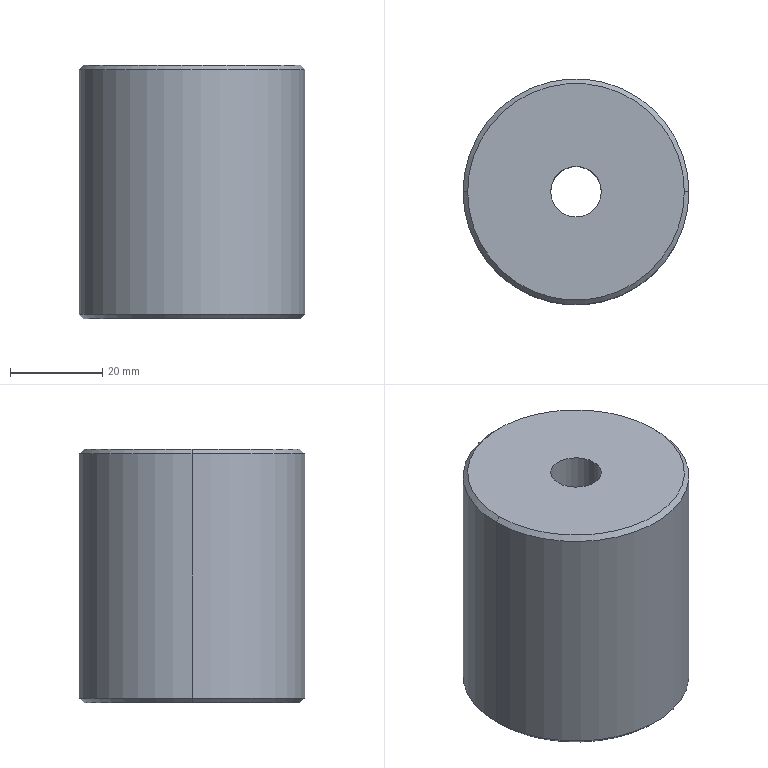Part | SolidWorks | features BaseBody 1 | 1 solid | 13 faces | box 49 x 49 x 55 mm | volume 96424 mm3 | cylinder 6 | cone 4 | plane 3 | commonest cylinder face diameters 11 x2 18 x2 49 x2
STEP:
#1=CARTESIAN_POINT('',(-196.5,115.,-210.5));
#2=VERTEX_POINT('',#1);
#3=CARTESIAN_POINT('',(-243.5,115.,-210.5));
#4=VERTEX_POINT('',#3);
#5=CARTESIAN_POINT('',(-220.,115.,-210.5));
#6=DIRECTION('',(0.,0.,1.));
#7=DIRECTION('',(1.,0.,0.));
#8=AXIS2_PLACEMENT_3D('',#5,#6,#7);
#9=CIRCLE('',#8,23.5);
#10=EDGE_CURVE('',#2,#4,#9,.T.);
#11=ORIENTED_EDGE('',*,*,#10,.F.);
#12=CARTESIAN_POINT('',(-195.5,115.,-211.5));
#13=VERTEX_POINT('',#12);
#14=CARTESIAN_POINT('',(-195.5,115.,-211.5));
#15=DIRECTION('',(0.7071,0.,-0.7071));
#16=VECTOR('',#15,1000.);
#17=LINE('',#14,#16);
#18=EDGE_CURVE('',#2,#13,#17,.T.);
#19=ORIENTED_EDGE('',*,*,#18,.T.);
#20=CARTESIAN_POINT('',(-244.5,115.,-211.5));
#21=VERTEX_POINT('',#20);
#22=CARTESIAN_POINT('',(-220.,115.,-211.5));
#23=DIRECTION('',(0.,0.,-1.));
#24=DIRECTION('',(1.,0.,0.));
#25=AXIS2_PLACEMENT_3D('',#22,#23,#24);
#26=CIRCLE('',#25,24.5);
#27=EDGE_CURVE('',#21,#13,#26,.T.);
#28=ORIENTED_EDGE('',*,*,#27,.F.);
#29=CARTESIAN_POINT('',(-244.5,115.,-211.5));
#30=DIRECTION('',(-0.7071,0.,-0.7071));
#31=VECTOR('',#30,1000.);
#32=LINE('',#29,#31);
#33=EDGE_CURVE('',#4,#21,#32,.T.);
#34=ORIENTED_EDGE('',*,*,#33,.F.);
#35=EDGE_LOOP('',(#11,#19,#28,#34));
#36=FACE_OUTER_BOUND('',#35,.T.);
#37=CARTESIAN_POINT('',(-220.,115.,-211.5));
#38=DIRECTION('',(0.,0.,-1.));
#39=DIRECTION('',(-1.,0.,0.));
#40=AXIS2_PLACEMENT_3D('',#37,#38,#39);
#41=CONICAL_SURFACE('',#40,24.5,0.7854);
#42=ADVANCED_FACE('',(#36),#41,.T.);
#43=CARTESIAN_POINT('',(-243.5,115.,-265.5));
#44=VERTEX_POINT('',#43);
#45=CARTESIAN_POINT('',(-196.5,115.,-265.5));
#46=VERTEX_POINT('',#45);
#47=CARTESIAN_POINT('',(-220.,115.,-265.5));
#48=DIRECTION('',(0.,0.,-1.));
#49=DIRECTION('',(-1.,0.,0.));
#50=AXIS2_PLACEMENT_3D('',#47,#48,#49);
#51=CIRCLE('',#50,23.5);
#52=EDGE_CURVE('',#44,#46,#51,.T.);
#53=ORIENTED_EDGE('',*,*,#52,.F.);
#54=CARTESIAN_POINT('',(-244.5,115.,-264.5));
#55=VERTEX_POINT('',#54);
#56=CARTESIAN_POINT('',(-244.5,115.,-264.5));
#57=DIRECTION('',(-0.7071,0.,0.7071));
#58=VECTOR('',#57,1000.);
#59=LINE('',#56,#58);
#60=EDGE_CURVE('',#44,#55,#59,.T.);
#61=ORIENTED_EDGE('',*,*,#60,.T.);
#62=CARTESIAN_POINT('',(-195.5,115.,-264.5));
#63=VERTEX_POINT('',#62);
#64=CARTESIAN_POINT('',(-220.,115.,-264.5));
#65=DIRECTION('',(0.,0.,1.));
#66=DIRECTION('',(-1.,0.,0.));
#67=AXIS2_PLACEMENT_3D('',#64,#65,#66);
#68=CIRCLE('',#67,24.5);
#69=EDGE_CURVE('',#63,#55,#68,.T.);
#70=ORIENTED_EDGE('',*,*,#69,.F.);
#71=CARTESIAN_POINT('',(-195.5,115.,-264.5));
#72=DIRECTION('',(0.7071,0.,0.7071));
#73=VECTOR('',#72,1000.);
#74=LINE('',#71,#73);
#75=EDGE_CURVE('',#46,#63,#74,.T.);
#76=ORIENTED_EDGE('',*,*,#75,.F.);
#77=EDGE_LOOP('',(#53,#61,#70,#76));
#78=FACE_OUTER_BOUND('',#77,.T.);
#79=CARTESIAN_POINT('',(-220.,115.,-264.5));
#80=DIRECTION('',(0.,0.,1.));
#81=DIRECTION('',(1.,0.,0.));
#82=AXIS2_PLACEMENT_3D('',#79,#80,#81);
#83=CONICAL_SURFACE('',#82,24.5,0.7854);
#84=ADVANCED_FACE('',(#78),#83,.T.);
#85=CARTESIAN_POINT('',(-229.,115.,-265.5));
#86=VERTEX_POINT('',#85);
#87=CARTESIAN_POINT('',(-211.,115.,-265.5));
#88=VERTEX_POINT('',#87);
#89=CARTESIAN_POINT('',(-220.,115.,-265.5));
#90=DIRECTION('',(0.,0.,-1.));
#91=DIRECTION('',(-1.,0.,0.));
#92=AXIS2_PLACEMENT_3D('',#89,#90,#91);
#93=CIRCLE('',#92,9.);
#94=EDGE_CURVE('',#86,#88,#93,.T.);
#95=ORIENTED_EDGE('',*,*,#94,.T.);
#96=CARTESIAN_POINT('',(-211.,115.,-253.5));
#97=VERTEX_POINT('',#96);
#98=CARTESIAN_POINT('',(-211.,115.,-265.5));
#99=DIRECTION('',(0.,0.,1.));
#100=VECTOR('',#99,1000.);
#101=LINE('',#98,#100);
#102=EDGE_CURVE('',#88,#97,#101,.T.);
#103=ORIENTED_EDGE('',*,*,#102,.T.);
#104=CARTESIAN_POINT('',(-229.,115.,-253.5));
#105=VERTEX_POINT('',#104);
#106=CARTESIAN_POINT('',(-220.,115.,-253.5));
#107=DIRECTION('',(0.,0.,-1.));
#108=DIRECTION('',(-1.,0.,0.));
#109=AXIS2_PLACEMENT_3D('',#106,#107,#108);
#110=CIRCLE('',#109,9.);
#111=EDGE_CURVE('',#105,#97,#110,.T.);
#112=ORIENTED_EDGE('',*,*,#111,.F.);
#113=CARTESIAN_POINT('',(-229.,115.,-265.5));
#114=DIRECTION('',(0.,0.,1.));
#115=VECTOR('',#114,1000.);
#116=LINE('',#113,#115);
#117=EDGE_CURVE('',#86,#105,#116,.T.);
#118=ORIENTED_EDGE('',*,*,#117,.F.);
#119=EDGE_LOOP('',(#95,#103,#112,#118));
#120=FACE_OUTER_BOUND('',#119,.T.);
#121=CARTESIAN_POINT('',(-220.,115.,-265.5));
#122=DIRECTION('',(0.,0.,1.));
#123=DIRECTION('',(-1.,0.,0.));
#124=AXIS2_PLACEMENT_3D('',#121,#122,#123);
#125=CYLINDRICAL_SURFACE('',#124,9.);
#126=ADVANCED_FACE('',(#120),#125,.F.);
#127=CARTESIAN_POINT('',(-214.5,115.,-253.5));
#128=VERTEX_POINT('',#127);
#129=CARTESIAN_POINT('',(-225.5,115.,-253.5));
#130=VERTEX_POINT('',#129);
#131=CARTESIAN_POINT('',(-220.,115.,-253.5));
#132=DIRECTION('',(0.,0.,1.));
#133=DIRECTION('',(-1.,0.,0.));
#134=AXIS2_PLACEMENT_3D('',#131,#132,#133);
#135=CIRCLE('',#134,5.5);
#136=EDGE_CURVE('',#128,#130,#135,.T.);
#137=ORIENTED_EDGE('',*,*,#136,.F.);
#138=CARTESIAN_POINT('',(-214.5,115.,-210.5));
#139=VERTEX_POINT('',#138);
#140=CARTESIAN_POINT('',(-214.5,115.,-265.5));
#141=DIRECTION('',(0.,0.,1.));
#142=VECTOR('',#141,1000.);
#143=LINE('',#140,#142);
#144=EDGE_CURVE('',#128,#139,#143,.T.);
#145=ORIENTED_EDGE('',*,*,#144,.T.);
#146=CARTESIAN_POINT('',(-225.5,115.,-210.5));
#147=VERTEX_POINT('',#146);
#148=CARTESIAN_POINT('',(-220.,115.,-210.5));
#149=DIRECTION('',(0.,0.,-1.));
#150=DIRECTION('',(1.,0.,0.));
#151=AXIS2_PLACEMENT_3D('',#148,#149,#150);
#152=CIRCLE('',#151,5.5);
#153=EDGE_CURVE('',#147,#139,#152,.T.);
#154=ORIENTED_EDGE('',*,*,#153,.F.);
#155=CARTESIAN_POINT('',(-225.5,115.,-265.5));
#156=DIRECTION('',(0.,0.,1.));
#157=VECTOR('',#156,1000.);
#158=LINE('',#155,#157);
#159=EDGE_CURVE('',#130,#147,#158,.T.);
#160=ORIENTED_EDGE('',*,*,#159,.F.);
#161=EDGE_LOOP('',(#137,#145,#154,#160));
#162=FACE_OUTER_BOUND('',#161,.T.);
#163=CARTESIAN_POINT('',(-220.,115.,-265.5));
#164=DIRECTION('',(0.,0.,1.));
#165=DIRECTION('',(-1.,0.,0.));
#166=AXIS2_PLACEMENT_3D('',#163,#164,#165);
#167=CYLINDRICAL_SURFACE('',#166,5.5);
#168=ADVANCED_FACE('',(#162),#167,.F.);
#169=CARTESIAN_POINT('',(-220.,115.,-211.5));
#170=DIRECTION('',(0.,0.,-1.));
#171=DIRECTION('',(1.,0.,0.));
#172=AXIS2_PLACEMENT_3D('',#169,#170,#171);
#173=CIRCLE('',#172,24.5);
#174=EDGE_CURVE('',#13,#21,#173,.T.);
#175=ORIENTED_EDGE('',*,*,#174,.T.);
#176=CARTESIAN_POINT('',(-244.5,115.,-165.5));
#177=DIRECTION('',(0.,0.,-1.));
#178=VECTOR('',#177,1000.);
#179=LINE('',#176,#178);
#180=EDGE_CURVE('',#21,#55,#179,.T.);
#181=ORIENTED_EDGE('',*,*,#180,.T.);
#182=CARTESIAN_POINT('',(-220.,115.,-264.5));
#183=DIRECTION('',(0.,0.,1.));
#184=DIRECTION('',(-1.,0.,0.));
#185=AXIS2_PLACEMENT_3D('',#182,#183,#184);
#186=CIRCLE('',#185,24.5);
#187=EDGE_CURVE('',#55,#63,#186,.T.);
#188=ORIENTED_EDGE('',*,*,#187,.T.);
#189=CARTESIAN_POINT('',(-195.5,115.,-165.5));
#190=DIRECTION('',(0.,0.,-1.));
#191=VECTOR('',#190,1000.);
#192=LINE('',#189,#191);
#193=EDGE_CURVE('',#13,#63,#192,.T.);
#194=ORIENTED_EDGE('',*,*,#193,.F.);
#195=EDGE_LOOP('',(#175,#181,#188,#194));
#196=FACE_OUTER_BOUND('',#195,.T.);
#197=CARTESIAN_POINT('',(-220.,115.,-165.5));
#198=DIRECTION('',(0.,0.,-1.));
#199=DIRECTION('',(1.,0.,0.));
#200=AXIS2_PLACEMENT_3D('',#197,#198,#199);
#201=CYLINDRICAL_SURFACE('',#200,24.5);
#202=ADVANCED_FACE('',(#196),#201,.T.);
#203=ORIENTED_EDGE('',*,*,#180,.F.);
#204=ORIENTED_EDGE('',*,*,#27,.T.);
#205=ORIENTED_EDGE('',*,*,#193,.T.);
#206=ORIENTED_EDGE('',*,*,#69,.T.);
#207=EDGE_LOOP('',(#203,#204,#205,#206));
#208=FACE_OUTER_BOUND('',#207,.T.);
#209=CARTESIAN_POINT('',(-220.,115.,-165.5));
#210=DIRECTION('',(0.,0.,-1.));
#211=DIRECTION('',(1.,0.,0.));
#212=AXIS2_PLACEMENT_3D('',#209,#210,#211);
#213=CYLINDRICAL_SURFACE('',#212,24.5);
#214=ADVANCED_FACE('',(#208),#213,.T.);
#215=CARTESIAN_POINT('',(-220.,115.,-210.5));
#216=DIRECTION('',(0.,0.,1.));
#217=DIRECTION('',(1.,0.,0.));
#218=AXIS2_PLACEMENT_3D('',#215,#216,#217);
#219=CIRCLE('',#218,23.5);
#220=EDGE_CURVE('',#4,#2,#219,.T.);
#221=ORIENTED_EDGE('',*,*,#220,.T.);
#222=ORIENTED_EDGE('',*,*,#10,.T.);
#223=EDGE_LOOP('',(#221,#222));
#224=FACE_OUTER_BOUND('',#223,.T.);
#225=ORIENTED_EDGE('',*,*,#153,.T.);
#226=CARTESIAN_POINT('',(-220.,115.,-210.5));
#227=DIRECTION('',(0.,0.,-1.));
#228=DIRECTION('',(1.,0.,0.));
#229=AXIS2_PLACEMENT_3D('',#226,#227,#228);
#230=CIRCLE('',#229,5.5);
#231=EDGE_CURVE('',#139,#147,#230,.T.);
#232=ORIENTED_EDGE('',*,*,#231,.T.);
#233=EDGE_LOOP('',(#225,#232));
#234=FACE_BOUND('',#233,.T.);
#235=CARTESIAN_POINT('',(-170.,-105.,-210.5));
#236=DIRECTION('',(0.,0.,1.));
#237=DIRECTION('',(1.,0.,0.));
#238=AXIS2_PLACEMENT_3D('',#235,#236,#237);
#239=PLANE('',#238);
#240=ADVANCED_FACE('',(#224,#234),#239,.T.);
#241=ORIENTED_EDGE('',*,*,#144,.F.);
#242=CARTESIAN_POINT('',(-220.,115.,-253.5));
#243=DIRECTION('',(0.,0.,1.));
#244=DIRECTION('',(-1.,0.,0.));
#245=AXIS2_PLACEMENT_3D('',#242,#243,#244);
#246=CIRCLE('',#245,5.5);
#247=EDGE_CURVE('',#130,#128,#246,.T.);
#248=ORIENTED_EDGE('',*,*,#247,.F.);
#249=ORIENTED_EDGE('',*,*,#159,.T.);
#250=ORIENTED_EDGE('',*,*,#231,.F.);
#251=EDGE_LOOP('',(#241,#248,#249,#250));
#252=FACE_OUTER_BOUND('',#251,.T.);
#253=CARTESIAN_POINT('',(-220.,115.,-265.5));
#254=DIRECTION('',(0.,0.,1.));
#255=DIRECTION('',(-1.,0.,0.));
#256=AXIS2_PLACEMENT_3D('',#253,#254,#255);
#257=CYLINDRICAL_SURFACE('',#256,5.5);
#258=ADVANCED_FACE('',(#252),#257,.F.);
#259=CARTESIAN_POINT('',(-220.,115.,-265.5));
#260=DIRECTION('',(0.,0.,-1.));
#261=DIRECTION('',(-1.,0.,0.));
#262=AXIS2_PLACEMENT_3D('',#259,#260,#261);
#263=CIRCLE('',#262,23.5);
#264=EDGE_CURVE('',#46,#44,#263,.T.);
#265=ORIENTED_EDGE('',*,*,#264,.T.);
#266=ORIENTED_EDGE('',*,*,#52,.T.);
#267=EDGE_LOOP('',(#265,#266));
#268=FACE_OUTER_BOUND('',#267,.T.);
#269=ORIENTED_EDGE('',*,*,#94,.F.);
#270=CARTESIAN_POINT('',(-220.,115.,-265.5));
#271=DIRECTION('',(0.,0.,-1.));
#272=DIRECTION('',(-1.,0.,0.));
#273=AXIS2_PLACEMENT_3D('',#270,#271,#272);
#274=CIRCLE('',#273,9.);
#275=EDGE_CURVE('',#88,#86,#274,.T.);
#276=ORIENTED_EDGE('',*,*,#275,.F.);
#277=EDGE_LOOP('',(#269,#276));
#278=FACE_BOUND('',#277,.T.);
#279=CARTESIAN_POINT('',(-220.,115.,-265.5));
#280=DIRECTION('',(0.,0.,-1.));
#281=DIRECTION('',(1.,0.,0.));
#282=AXIS2_PLACEMENT_3D('',#279,#280,#281);
#283=PLANE('',#282);
#284=ADVANCED_FACE('',(#268,#278),#283,.T.);
#285=ORIENTED_EDGE('',*,*,#111,.T.);
#286=CARTESIAN_POINT('',(-220.,115.,-253.5));
#287=DIRECTION('',(0.,0.,-1.));
#288=DIRECTION('',(-1.,0.,0.));
#289=AXIS2_PLACEMENT_3D('',#286,#287,#288);
#290=CIRCLE('',#289,9.);
#291=EDGE_CURVE('',#97,#105,#290,.T.);
#292=ORIENTED_EDGE('',*,*,#291,.T.);
#293=EDGE_LOOP('',(#285,#292));
#294=FACE_OUTER_BOUND('',#293,.T.);
#295=ORIENTED_EDGE('',*,*,#247,.T.);
#296=ORIENTED_EDGE('',*,*,#136,.T.);
#297=EDGE_LOOP('',(#295,#296));
#298=FACE_BOUND('',#297,.T.);
#299=CARTESIAN_POINT('',(-220.,115.,-253.5));
#300=DIRECTION('',(0.,0.,1.));
#301=DIRECTION('',(-1.,0.,0.));
#302=AXIS2_PLACEMENT_3D('',#299,#300,#301);
#303=PLANE('',#302);
#304=ADVANCED_FACE('',(#294,#298),#303,.F.);
#305=ORIENTED_EDGE('',*,*,#102,.F.);
#306=ORIENTED_EDGE('',*,*,#275,.T.);
#307=ORIENTED_EDGE('',*,*,#117,.T.);
#308=ORIENTED_EDGE('',*,*,#291,.F.);
#309=EDGE_LOOP('',(#305,#306,#307,#308));
#310=FACE_OUTER_BOUND('',#309,.T.);
#311=CARTESIAN_POINT('',(-220.,115.,-265.5));
#312=DIRECTION('',(0.,0.,1.));
#313=DIRECTION('',(-1.,0.,0.));
#314=AXIS2_PLACEMENT_3D('',#311,#312,#313);
#315=CYLINDRICAL_SURFACE('',#314,9.);
#316=ADVANCED_FACE('',(#310),#315,.F.);
#317=ORIENTED_EDGE('',*,*,#60,.F.);
#318=ORIENTED_EDGE('',*,*,#264,.F.);
#319=ORIENTED_EDGE('',*,*,#75,.T.);
#320=ORIENTED_EDGE('',*,*,#187,.F.);
#321=EDGE_LOOP('',(#317,#318,#319,#320));
#322=FACE_OUTER_BOUND('',#321,.T.);
#323=CARTESIAN_POINT('',(-220.,115.,-264.5));
#324=DIRECTION('',(0.,0.,1.));
#325=DIRECTION('',(1.,0.,0.));
#326=AXIS2_PLACEMENT_3D('',#323,#324,#325);
#327=CONICAL_SURFACE('',#326,24.5,0.7854);
#328=ADVANCED_FACE('',(#322),#327,.T.);
#329=ORIENTED_EDGE('',*,*,#18,.F.);
#330=ORIENTED_EDGE('',*,*,#220,.F.);
#331=ORIENTED_EDGE('',*,*,#33,.T.);
#332=ORIENTED_EDGE('',*,*,#174,.F.);
#333=EDGE_LOOP('',(#329,#330,#331,#332));
#334=FACE_OUTER_BOUND('',#333,.T.);
#335=CARTESIAN_POINT('',(-220.,115.,-211.5));
#336=DIRECTION('',(0.,0.,-1.));
#337=DIRECTION('',(-1.,0.,0.));
#338=AXIS2_PLACEMENT_3D('',#335,#336,#337);
#339=CONICAL_SURFACE('',#338,24.5,0.7854);
#340=ADVANCED_FACE('',(#334),#339,.T.);
#341=CLOSED_SHELL('',(#42,#84,#126,#168,#202,#214,#240,#258,#284,#304,#316,#328,#340));
#342=MANIFOLD_SOLID_BREP('',#341);
#343=CARTESIAN_POINT('',(0.,0.,0.));
#344=DIRECTION('',(0.,0.,1.));
#345=DIRECTION('',(1.,0.,0.));
#346=AXIS2_PLACEMENT_3D('',#343,#344,#345);
#347=(LENGTH_UNIT()NAMED_UNIT(*)SI_UNIT(.MILLI.,.METRE.));
#348=UNCERTAINTY_MEASURE_WITH_UNIT(LENGTH_MEASURE(0.00001),#347,'','');
#349=(NAMED_UNIT(*)PLANE_ANGLE_UNIT()SI_UNIT($,.RADIAN.));
#350=(NAMED_UNIT(*)SI_UNIT($,.STERADIAN.)SOLID_ANGLE_UNIT());
#351=(GEOMETRIC_REPRESENTATION_CONTEXT(3)GLOBAL_UNCERTAINTY_ASSIGNED_CONTEXT((#348))GLOBAL_UNIT_ASSIGNED_CONTEXT((#347,#349,#350))REPRESENTATION_CONTEXT('',''));
#352=ADVANCED_BREP_SHAPE_REPRESENTATION('',(#342,#346),#351);